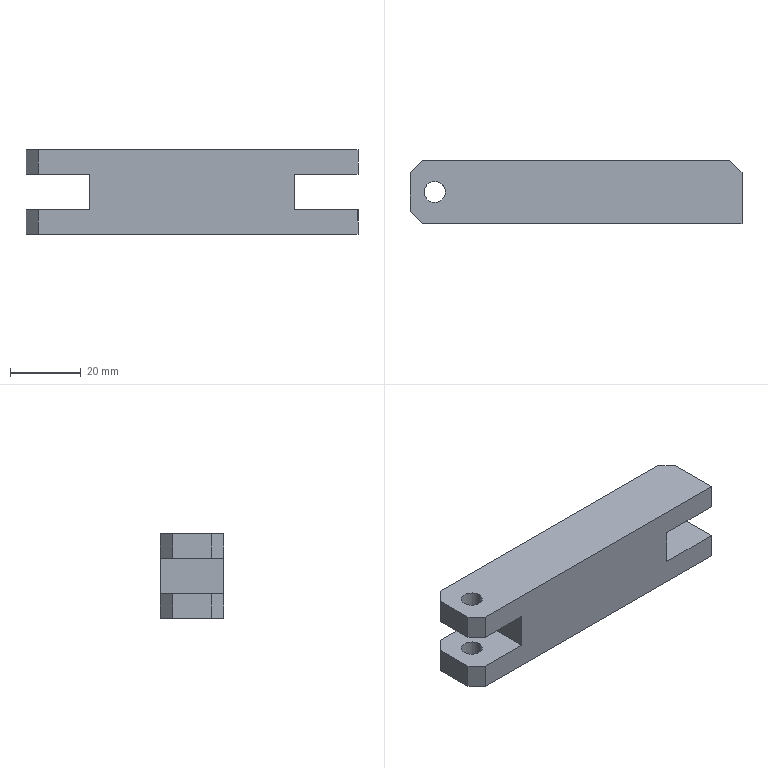Part | SolidWorks | features Chamfer 2, ICE 2, Extrusion 1 | 1 solid | 24 faces | box 94 x 18 x 24 mm | volume 33475 mm3 | plane 20 | cylinder 4 | commonest cylinder face diameters 6 x4
STEP:
#1=CARTESIAN_POINT('',(-43.,9.,5.));
#2=VERTEX_POINT('',#1);
#3=CARTESIAN_POINT('',(-37.,9.,5.));
#4=VERTEX_POINT('',#3);
#5=CARTESIAN_POINT('',(-40.,9.,5.));
#6=DIRECTION('',(0.,0.,1.));
#7=DIRECTION('',(1.,0.,0.));
#8=AXIS2_PLACEMENT_3D('',#5,#6,#7);
#9=CIRCLE('',#8,3.);
#10=EDGE_CURVE('',#2,#4,#9,.T.);
#11=ORIENTED_EDGE('',*,*,#10,.F.);
#12=CARTESIAN_POINT('',(-43.,9.,12.));
#13=VERTEX_POINT('',#12);
#14=CARTESIAN_POINT('',(-43.,9.,-58.));
#15=DIRECTION('',(0.,0.,1.));
#16=VECTOR('',#15,1000.);
#17=LINE('',#14,#16);
#18=EDGE_CURVE('',#2,#13,#17,.T.);
#19=ORIENTED_EDGE('',*,*,#18,.T.);
#20=CARTESIAN_POINT('',(-37.,9.,12.));
#21=VERTEX_POINT('',#20);
#22=CARTESIAN_POINT('',(-40.,9.,12.));
#23=DIRECTION('',(0.,0.,1.));
#24=DIRECTION('',(1.,0.,0.));
#25=AXIS2_PLACEMENT_3D('',#22,#23,#24);
#26=CIRCLE('',#25,3.);
#27=EDGE_CURVE('',#13,#21,#26,.T.);
#28=ORIENTED_EDGE('',*,*,#27,.T.);
#29=CARTESIAN_POINT('',(-37.,9.,-58.));
#30=DIRECTION('',(0.,0.,1.));
#31=VECTOR('',#30,1000.);
#32=LINE('',#29,#31);
#33=EDGE_CURVE('',#4,#21,#32,.T.);
#34=ORIENTED_EDGE('',*,*,#33,.F.);
#35=EDGE_LOOP('',(#11,#19,#28,#34));
#36=FACE_OUTER_BOUND('',#35,.T.);
#37=CARTESIAN_POINT('',(-40.,9.,-58.));
#38=DIRECTION('',(0.,0.,1.));
#39=DIRECTION('',(1.,0.,0.));
#40=AXIS2_PLACEMENT_3D('',#37,#38,#39);
#41=CYLINDRICAL_SURFACE('',#40,3.);
#42=ADVANCED_FACE('',(#36),#41,.F.);
#43=CARTESIAN_POINT('',(-43.,9.,-12.));
#44=VERTEX_POINT('',#43);
#45=CARTESIAN_POINT('',(-37.,9.,-12.));
#46=VERTEX_POINT('',#45);
#47=CARTESIAN_POINT('',(-40.,9.,-12.));
#48=DIRECTION('',(0.,0.,1.));
#49=DIRECTION('',(1.,0.,0.));
#50=AXIS2_PLACEMENT_3D('',#47,#48,#49);
#51=CIRCLE('',#50,3.);
#52=EDGE_CURVE('',#44,#46,#51,.T.);
#53=ORIENTED_EDGE('',*,*,#52,.F.);
#54=CARTESIAN_POINT('',(-43.,9.,-5.));
#55=VERTEX_POINT('',#54);
#56=CARTESIAN_POINT('',(-43.,9.,-58.));
#57=DIRECTION('',(0.,0.,1.));
#58=VECTOR('',#57,1000.);
#59=LINE('',#56,#58);
#60=EDGE_CURVE('',#44,#55,#59,.T.);
#61=ORIENTED_EDGE('',*,*,#60,.T.);
#62=CARTESIAN_POINT('',(-37.,9.,-5.));
#63=VERTEX_POINT('',#62);
#64=CARTESIAN_POINT('',(-40.,9.,-5.));
#65=DIRECTION('',(0.,0.,-1.));
#66=DIRECTION('',(-1.,0.,0.));
#67=AXIS2_PLACEMENT_3D('',#64,#65,#66);
#68=CIRCLE('',#67,3.);
#69=EDGE_CURVE('',#63,#55,#68,.T.);
#70=ORIENTED_EDGE('',*,*,#69,.F.);
#71=CARTESIAN_POINT('',(-37.,9.,-58.));
#72=DIRECTION('',(0.,0.,1.));
#73=VECTOR('',#72,1000.);
#74=LINE('',#71,#73);
#75=EDGE_CURVE('',#46,#63,#74,.T.);
#76=ORIENTED_EDGE('',*,*,#75,.F.);
#77=EDGE_LOOP('',(#53,#61,#70,#76));
#78=FACE_OUTER_BOUND('',#77,.T.);
#79=CARTESIAN_POINT('',(-40.,9.,-58.));
#80=DIRECTION('',(0.,0.,1.));
#81=DIRECTION('',(1.,0.,0.));
#82=AXIS2_PLACEMENT_3D('',#79,#80,#81);
#83=CYLINDRICAL_SURFACE('',#82,3.);
#84=ADVANCED_FACE('',(#78),#83,.F.);
#85=CARTESIAN_POINT('',(47.,0.,5.));
#86=VERTEX_POINT('',#85);
#87=CARTESIAN_POINT('',(47.,14.5,5.));
#88=VERTEX_POINT('',#87);
#89=CARTESIAN_POINT('',(47.,18.,5.));
#90=DIRECTION('',(0.,1.,0.));
#91=VECTOR('',#90,1000.);
#92=LINE('',#89,#91);
#93=EDGE_CURVE('',#86,#88,#92,.T.);
#94=ORIENTED_EDGE('',*,*,#93,.T.);
#95=CARTESIAN_POINT('',(47.,14.5,12.));
#96=VERTEX_POINT('',#95);
#97=CARTESIAN_POINT('',(47.,14.5,12.));
#98=DIRECTION('',(0.,0.,1.));
#99=VECTOR('',#98,1000.);
#100=LINE('',#97,#99);
#101=EDGE_CURVE('',#88,#96,#100,.T.);
#102=ORIENTED_EDGE('',*,*,#101,.T.);
#103=CARTESIAN_POINT('',(47.,0.,12.));
#104=VERTEX_POINT('',#103);
#105=CARTESIAN_POINT('',(47.,18.,12.));
#106=DIRECTION('',(0.,-1.,0.));
#107=VECTOR('',#106,1000.);
#108=LINE('',#105,#107);
#109=EDGE_CURVE('',#96,#104,#108,.T.);
#110=ORIENTED_EDGE('',*,*,#109,.T.);
#111=CARTESIAN_POINT('',(47.,0.,-12.));
#112=DIRECTION('',(0.,0.,-1.));
#113=VECTOR('',#112,1000.);
#114=LINE('',#111,#113);
#115=EDGE_CURVE('',#104,#86,#114,.T.);
#116=ORIENTED_EDGE('',*,*,#115,.T.);
#117=EDGE_LOOP('',(#94,#102,#110,#116));
#118=FACE_OUTER_BOUND('',#117,.T.);
#119=CARTESIAN_POINT('',(47.,18.,-12.));
#120=DIRECTION('',(-1.,0.,0.));
#121=DIRECTION('',(0.,0.,1.));
#122=AXIS2_PLACEMENT_3D('',#119,#120,#121);
#123=PLANE('',#122);
#124=ADVANCED_FACE('',(#118),#123,.F.);
#125=CARTESIAN_POINT('',(-47.,14.5,5.));
#126=VERTEX_POINT('',#125);
#127=CARTESIAN_POINT('',(-47.,3.5,5.));
#128=VERTEX_POINT('',#127);
#129=CARTESIAN_POINT('',(-47.,18.,5.));
#130=DIRECTION('',(0.,-1.,0.));
#131=VECTOR('',#130,1000.);
#132=LINE('',#129,#131);
#133=EDGE_CURVE('',#126,#128,#132,.T.);
#134=ORIENTED_EDGE('',*,*,#133,.T.);
#135=CARTESIAN_POINT('',(-47.,3.5,12.));
#136=VERTEX_POINT('',#135);
#137=CARTESIAN_POINT('',(-47.,3.5,-12.));
#138=DIRECTION('',(0.,0.,1.));
#139=VECTOR('',#138,1000.);
#140=LINE('',#137,#139);
#141=EDGE_CURVE('',#128,#136,#140,.T.);
#142=ORIENTED_EDGE('',*,*,#141,.T.);
#143=CARTESIAN_POINT('',(-47.,14.5,12.));
#144=VERTEX_POINT('',#143);
#145=CARTESIAN_POINT('',(-47.,18.,12.));
#146=DIRECTION('',(0.,-1.,0.));
#147=VECTOR('',#146,1000.);
#148=LINE('',#145,#147);
#149=EDGE_CURVE('',#144,#136,#148,.T.);
#150=ORIENTED_EDGE('',*,*,#149,.F.);
#151=CARTESIAN_POINT('',(-47.,14.5,5.));
#152=DIRECTION('',(0.,0.,-1.));
#153=VECTOR('',#152,1000.);
#154=LINE('',#151,#153);
#155=EDGE_CURVE('',#144,#126,#154,.T.);
#156=ORIENTED_EDGE('',*,*,#155,.T.);
#157=EDGE_LOOP('',(#134,#142,#150,#156));
#158=FACE_OUTER_BOUND('',#157,.T.);
#159=CARTESIAN_POINT('',(-47.,18.,-12.));
#160=DIRECTION('',(1.,0.,0.));
#161=DIRECTION('',(0.,0.,-1.));
#162=AXIS2_PLACEMENT_3D('',#159,#160,#161);
#163=PLANE('',#162);
#164=ADVANCED_FACE('',(#158),#163,.F.);
#165=CARTESIAN_POINT('',(47.,14.5,-12.));
#166=VERTEX_POINT('',#165);
#167=CARTESIAN_POINT('',(47.,0.,-12.));
#168=VERTEX_POINT('',#167);
#169=CARTESIAN_POINT('',(47.,18.,-12.));
#170=DIRECTION('',(0.,-1.,0.));
#171=VECTOR('',#170,1000.);
#172=LINE('',#169,#171);
#173=EDGE_CURVE('',#166,#168,#172,.T.);
#174=ORIENTED_EDGE('',*,*,#173,.F.);
#175=CARTESIAN_POINT('',(47.,14.5,-5.));
#176=VERTEX_POINT('',#175);
#177=CARTESIAN_POINT('',(47.,14.5,-5.));
#178=DIRECTION('',(0.,0.,1.));
#179=VECTOR('',#178,1000.);
#180=LINE('',#177,#179);
#181=EDGE_CURVE('',#166,#176,#180,.T.);
#182=ORIENTED_EDGE('',*,*,#181,.T.);
#183=CARTESIAN_POINT('',(47.,0.,-5.));
#184=VERTEX_POINT('',#183);
#185=CARTESIAN_POINT('',(47.,18.,-5.));
#186=DIRECTION('',(0.,-1.,0.));
#187=VECTOR('',#186,1000.);
#188=LINE('',#185,#187);
#189=EDGE_CURVE('',#176,#184,#188,.T.);
#190=ORIENTED_EDGE('',*,*,#189,.T.);
#191=CARTESIAN_POINT('',(47.,0.,-12.));
#192=DIRECTION('',(0.,0.,-1.));
#193=VECTOR('',#192,1000.);
#194=LINE('',#191,#193);
#195=EDGE_CURVE('',#184,#168,#194,.T.);
#196=ORIENTED_EDGE('',*,*,#195,.T.);
#197=EDGE_LOOP('',(#174,#182,#190,#196));
#198=FACE_OUTER_BOUND('',#197,.T.);
#199=CARTESIAN_POINT('',(47.,18.,-12.));
#200=DIRECTION('',(-1.,0.,0.));
#201=DIRECTION('',(0.,0.,1.));
#202=AXIS2_PLACEMENT_3D('',#199,#200,#201);
#203=PLANE('',#202);
#204=ADVANCED_FACE('',(#198),#203,.F.);
#205=CARTESIAN_POINT('',(-40.,9.,-12.));
#206=DIRECTION('',(0.,0.,1.));
#207=DIRECTION('',(1.,0.,0.));
#208=AXIS2_PLACEMENT_3D('',#205,#206,#207);
#209=CIRCLE('',#208,3.);
#210=EDGE_CURVE('',#46,#44,#209,.T.);
#211=ORIENTED_EDGE('',*,*,#210,.T.);
#212=ORIENTED_EDGE('',*,*,#52,.T.);
#213=EDGE_LOOP('',(#211,#212));
#214=FACE_BOUND('',#213,.T.);
#215=CARTESIAN_POINT('',(-43.5,0.,-12.));
#216=VERTEX_POINT('',#215);
#217=CARTESIAN_POINT('',(-47.,0.,-12.));
#218=DIRECTION('',(-1.,0.,0.));
#219=VECTOR('',#218,1000.);
#220=LINE('',#217,#219);
#221=EDGE_CURVE('',#168,#216,#220,.T.);
#222=ORIENTED_EDGE('',*,*,#221,.T.);
#223=CARTESIAN_POINT('',(-47.,3.5,-12.));
#224=VERTEX_POINT('',#223);
#225=CARTESIAN_POINT('',(-47.,3.5,-12.));
#226=DIRECTION('',(-0.7071,0.7071,0.));
#227=VECTOR('',#226,1000.);
#228=LINE('',#225,#227);
#229=EDGE_CURVE('',#216,#224,#228,.T.);
#230=ORIENTED_EDGE('',*,*,#229,.T.);
#231=CARTESIAN_POINT('',(-47.,14.5,-12.));
#232=VERTEX_POINT('',#231);
#233=CARTESIAN_POINT('',(-47.,18.,-12.));
#234=DIRECTION('',(0.,-1.,0.));
#235=VECTOR('',#234,1000.);
#236=LINE('',#233,#235);
#237=EDGE_CURVE('',#232,#224,#236,.T.);
#238=ORIENTED_EDGE('',*,*,#237,.F.);
#239=CARTESIAN_POINT('',(-43.5,18.,-12.));
#240=VERTEX_POINT('',#239);
#241=CARTESIAN_POINT('',(-43.5,18.,-12.));
#242=DIRECTION('',(0.7071,0.7071,0.));
#243=VECTOR('',#242,1000.);
#244=LINE('',#241,#243);
#245=EDGE_CURVE('',#232,#240,#244,.T.);
#246=ORIENTED_EDGE('',*,*,#245,.T.);
#247=CARTESIAN_POINT('',(43.5,18.,-12.));
#248=VERTEX_POINT('',#247);
#249=CARTESIAN_POINT('',(-47.,18.,-12.));
#250=DIRECTION('',(-1.,0.,0.));
#251=VECTOR('',#250,1000.);
#252=LINE('',#249,#251);
#253=EDGE_CURVE('',#248,#240,#252,.T.);
#254=ORIENTED_EDGE('',*,*,#253,.F.);
#255=CARTESIAN_POINT('',(43.5,18.,-12.));
#256=DIRECTION('',(0.7071,-0.7071,0.));
#257=VECTOR('',#256,1000.);
#258=LINE('',#255,#257);
#259=EDGE_CURVE('',#248,#166,#258,.T.);
#260=ORIENTED_EDGE('',*,*,#259,.T.);
#261=ORIENTED_EDGE('',*,*,#173,.T.);
#262=EDGE_LOOP('',(#222,#230,#238,#246,#254,#260,#261));
#263=FACE_OUTER_BOUND('',#262,.T.);
#264=CARTESIAN_POINT('',(-47.,18.,-12.));
#265=DIRECTION('',(0.,0.,1.));
#266=DIRECTION('',(1.,0.,0.));
#267=AXIS2_PLACEMENT_3D('',#264,#265,#266);
#268=PLANE('',#267);
#269=ADVANCED_FACE('',(#214,#263),#268,.F.);
#270=ORIENTED_EDGE('',*,*,#237,.T.);
#271=CARTESIAN_POINT('',(-47.,3.5,-5.));
#272=VERTEX_POINT('',#271);
#273=CARTESIAN_POINT('',(-47.,3.5,-12.));
#274=DIRECTION('',(0.,0.,1.));
#275=VECTOR('',#274,1000.);
#276=LINE('',#273,#275);
#277=EDGE_CURVE('',#224,#272,#276,.T.);
#278=ORIENTED_EDGE('',*,*,#277,.T.);
#279=CARTESIAN_POINT('',(-47.,14.5,-5.));
#280=VERTEX_POINT('',#279);
#281=CARTESIAN_POINT('',(-47.,18.,-5.));
#282=DIRECTION('',(0.,1.,0.));
#283=VECTOR('',#282,1000.);
#284=LINE('',#281,#283);
#285=EDGE_CURVE('',#272,#280,#284,.T.);
#286=ORIENTED_EDGE('',*,*,#285,.T.);
#287=CARTESIAN_POINT('',(-47.,14.5,-12.));
#288=DIRECTION('',(0.,0.,-1.));
#289=VECTOR('',#288,1000.);
#290=LINE('',#287,#289);
#291=EDGE_CURVE('',#280,#232,#290,.T.);
#292=ORIENTED_EDGE('',*,*,#291,.T.);
#293=EDGE_LOOP('',(#270,#278,#286,#292));
#294=FACE_OUTER_BOUND('',#293,.T.);
#295=CARTESIAN_POINT('',(-47.,18.,-12.));
#296=DIRECTION('',(1.,0.,0.));
#297=DIRECTION('',(0.,0.,-1.));
#298=AXIS2_PLACEMENT_3D('',#295,#296,#297);
#299=PLANE('',#298);
#300=ADVANCED_FACE('',(#294),#299,.F.);
#301=CARTESIAN_POINT('',(-40.,9.,12.));
#302=DIRECTION('',(0.,0.,1.));
#303=DIRECTION('',(1.,0.,0.));
#304=AXIS2_PLACEMENT_3D('',#301,#302,#303);
#305=CIRCLE('',#304,3.);
#306=EDGE_CURVE('',#21,#13,#305,.T.);
#307=ORIENTED_EDGE('',*,*,#306,.F.);
#308=ORIENTED_EDGE('',*,*,#27,.F.);
#309=EDGE_LOOP('',(#307,#308));
#310=FACE_BOUND('',#309,.T.);
#311=ORIENTED_EDGE('',*,*,#149,.T.);
#312=CARTESIAN_POINT('',(-43.5,0.,12.));
#313=VERTEX_POINT('',#312);
#314=CARTESIAN_POINT('',(-47.,3.5,12.));
#315=DIRECTION('',(0.7071,-0.7071,0.));
#316=VECTOR('',#315,1000.);
#317=LINE('',#314,#316);
#318=EDGE_CURVE('',#136,#313,#317,.T.);
#319=ORIENTED_EDGE('',*,*,#318,.T.);
#320=CARTESIAN_POINT('',(-47.,0.,12.));
#321=DIRECTION('',(1.,0.,0.));
#322=VECTOR('',#321,1000.);
#323=LINE('',#320,#322);
#324=EDGE_CURVE('',#313,#104,#323,.T.);
#325=ORIENTED_EDGE('',*,*,#324,.T.);
#326=ORIENTED_EDGE('',*,*,#109,.F.);
#327=CARTESIAN_POINT('',(43.5,18.,12.));
#328=VERTEX_POINT('',#327);
#329=CARTESIAN_POINT('',(43.5,18.,12.));
#330=DIRECTION('',(-0.7071,0.7071,0.));
#331=VECTOR('',#330,1000.);
#332=LINE('',#329,#331);
#333=EDGE_CURVE('',#96,#328,#332,.T.);
#334=ORIENTED_EDGE('',*,*,#333,.T.);
#335=CARTESIAN_POINT('',(-43.5,18.,12.));
#336=VERTEX_POINT('',#335);
#337=CARTESIAN_POINT('',(-47.,18.,12.));
#338=DIRECTION('',(1.,0.,0.));
#339=VECTOR('',#338,1000.);
#340=LINE('',#337,#339);
#341=EDGE_CURVE('',#336,#328,#340,.T.);
#342=ORIENTED_EDGE('',*,*,#341,.F.);
#343=CARTESIAN_POINT('',(-43.5,18.,12.));
#344=DIRECTION('',(-0.7071,-0.7071,0.));
#345=VECTOR('',#344,1000.);
#346=LINE('',#343,#345);
#347=EDGE_CURVE('',#336,#144,#346,.T.);
#348=ORIENTED_EDGE('',*,*,#347,.T.);
#349=EDGE_LOOP('',(#311,#319,#325,#326,#334,#342,#348));
#350=FACE_OUTER_BOUND('',#349,.T.);
#351=CARTESIAN_POINT('',(-47.,18.,12.));
#352=DIRECTION('',(0.,0.,-1.));
#353=DIRECTION('',(-1.,0.,0.));
#354=AXIS2_PLACEMENT_3D('',#351,#352,#353);
#355=PLANE('',#354);
#356=ADVANCED_FACE('',(#310,#350),#355,.F.);
#357=ORIENTED_EDGE('',*,*,#253,.T.);
#358=CARTESIAN_POINT('',(-43.5,18.,-5.));
#359=VERTEX_POINT('',#358);
#360=CARTESIAN_POINT('',(-43.5,18.,-5.));
#361=DIRECTION('',(0.,0.,1.));
#362=VECTOR('',#361,1000.);
#363=LINE('',#360,#362);
#364=EDGE_CURVE('',#240,#359,#363,.T.);
#365=ORIENTED_EDGE('',*,*,#364,.T.);
#366=CARTESIAN_POINT('',(-29.,18.,-5.));
#367=VERTEX_POINT('',#366);
#368=CARTESIAN_POINT('',(-65.,18.,-5.));
#369=DIRECTION('',(-1.,0.,0.));
#370=VECTOR('',#369,1000.);
#371=LINE('',#368,#370);
#372=EDGE_CURVE('',#367,#359,#371,.T.);
#373=ORIENTED_EDGE('',*,*,#372,.F.);
#374=CARTESIAN_POINT('',(-29.,18.,5.));
#375=VERTEX_POINT('',#374);
#376=CARTESIAN_POINT('',(-29.,18.,-5.));
#377=DIRECTION('',(0.,0.,-1.));
#378=VECTOR('',#377,1000.);
#379=LINE('',#376,#378);
#380=EDGE_CURVE('',#375,#367,#379,.T.);
#381=ORIENTED_EDGE('',*,*,#380,.F.);
#382=CARTESIAN_POINT('',(-43.5,18.,5.));
#383=VERTEX_POINT('',#382);
#384=CARTESIAN_POINT('',(-65.,18.,5.));
#385=DIRECTION('',(1.,0.,0.));
#386=VECTOR('',#385,1000.);
#387=LINE('',#384,#386);
#388=EDGE_CURVE('',#383,#375,#387,.T.);
#389=ORIENTED_EDGE('',*,*,#388,.F.);
#390=CARTESIAN_POINT('',(-43.5,18.,12.));
#391=DIRECTION('',(0.,0.,1.));
#392=VECTOR('',#391,1000.);
#393=LINE('',#390,#392);
#394=EDGE_CURVE('',#383,#336,#393,.T.);
#395=ORIENTED_EDGE('',*,*,#394,.T.);
#396=ORIENTED_EDGE('',*,*,#341,.T.);
#397=CARTESIAN_POINT('',(43.5,18.,5.));
#398=VERTEX_POINT('',#397);
#399=CARTESIAN_POINT('',(43.5,18.,5.));
#400=DIRECTION('',(0.,0.,-1.));
#401=VECTOR('',#400,1000.);
#402=LINE('',#399,#401);
#403=EDGE_CURVE('',#328,#398,#402,.T.);
#404=ORIENTED_EDGE('',*,*,#403,.T.);
#405=CARTESIAN_POINT('',(29.,18.,5.));
#406=VERTEX_POINT('',#405);
#407=CARTESIAN_POINT('',(65.,18.,5.));
#408=DIRECTION('',(1.,0.,0.));
#409=VECTOR('',#408,1000.);
#410=LINE('',#407,#409);
#411=EDGE_CURVE('',#406,#398,#410,.T.);
#412=ORIENTED_EDGE('',*,*,#411,.F.);
#413=CARTESIAN_POINT('',(29.,18.,-5.));
#414=VERTEX_POINT('',#413);
#415=CARTESIAN_POINT('',(29.,18.,-5.));
#416=DIRECTION('',(0.,0.,1.));
#417=VECTOR('',#416,1000.);
#418=LINE('',#415,#417);
#419=EDGE_CURVE('',#414,#406,#418,.T.);
#420=ORIENTED_EDGE('',*,*,#419,.F.);
#421=CARTESIAN_POINT('',(43.5,18.,-5.));
#422=VERTEX_POINT('',#421);
#423=CARTESIAN_POINT('',(65.,18.,-5.));
#424=DIRECTION('',(-1.,0.,0.));
#425=VECTOR('',#424,1000.);
#426=LINE('',#423,#425);
#427=EDGE_CURVE('',#422,#414,#426,.T.);
#428=ORIENTED_EDGE('',*,*,#427,.F.);
#429=CARTESIAN_POINT('',(43.5,18.,-12.));
#430=DIRECTION('',(0.,0.,-1.));
#431=VECTOR('',#430,1000.);
#432=LINE('',#429,#431);
#433=EDGE_CURVE('',#422,#248,#432,.T.);
#434=ORIENTED_EDGE('',*,*,#433,.T.);
#435=EDGE_LOOP('',(#357,#365,#373,#381,#389,#395,#396,#404,#412,#420,#428,#434));
#436=FACE_OUTER_BOUND('',#435,.T.);
#437=CARTESIAN_POINT('',(47.,18.,12.));
#438=DIRECTION('',(0.,1.,0.));
#439=DIRECTION('',(0.,0.,1.));
#440=AXIS2_PLACEMENT_3D('',#437,#438,#439);
#441=PLANE('',#440);
#442=ADVANCED_FACE('',(#436),#441,.T.);
#443=ORIENTED_EDGE('',*,*,#324,.F.);
#444=CARTESIAN_POINT('',(-43.5,0.,5.));
#445=VERTEX_POINT('',#444);
#446=CARTESIAN_POINT('',(-43.5,0.,12.));
#447=DIRECTION('',(0.,0.,-1.));
#448=VECTOR('',#447,1000.);
#449=LINE('',#446,#448);
#450=EDGE_CURVE('',#313,#445,#449,.T.);
#451=ORIENTED_EDGE('',*,*,#450,.T.);
#452=CARTESIAN_POINT('',(-29.,0.,5.));
#453=VERTEX_POINT('',#452);
#454=CARTESIAN_POINT('',(47.,0.,5.));
#455=DIRECTION('',(1.,0.,0.));
#456=VECTOR('',#455,1000.);
#457=LINE('',#454,#456);
#458=EDGE_CURVE('',#445,#453,#457,.T.);
#459=ORIENTED_EDGE('',*,*,#458,.T.);
#460=CARTESIAN_POINT('',(-29.,0.,-5.));
#461=VERTEX_POINT('',#460);
#462=CARTESIAN_POINT('',(-29.,0.,12.));
#463=DIRECTION('',(0.,0.,-1.));
#464=VECTOR('',#463,1000.);
#465=LINE('',#462,#464);
#466=EDGE_CURVE('',#453,#461,#465,.T.);
#467=ORIENTED_EDGE('',*,*,#466,.T.);
#468=CARTESIAN_POINT('',(-43.5,0.,-5.));
#469=VERTEX_POINT('',#468);
#470=CARTESIAN_POINT('',(47.,0.,-5.));
#471=DIRECTION('',(-1.,0.,0.));
#472=VECTOR('',#471,1000.);
#473=LINE('',#470,#472);
#474=EDGE_CURVE('',#461,#469,#473,.T.);
#475=ORIENTED_EDGE('',*,*,#474,.T.);
#476=CARTESIAN_POINT('',(-43.5,0.,12.));
#477=DIRECTION('',(0.,0.,-1.));
#478=VECTOR('',#477,1000.);
#479=LINE('',#476,#478);
#480=EDGE_CURVE('',#469,#216,#479,.T.);
#481=ORIENTED_EDGE('',*,*,#480,.T.);
#482=ORIENTED_EDGE('',*,*,#221,.F.);
#483=ORIENTED_EDGE('',*,*,#195,.F.);
#484=CARTESIAN_POINT('',(29.,0.,-5.));
#485=VERTEX_POINT('',#484);
#486=CARTESIAN_POINT('',(47.,0.,-5.));
#487=DIRECTION('',(-1.,0.,0.));
#488=VECTOR('',#487,1000.);
#489=LINE('',#486,#488);
#490=EDGE_CURVE('',#184,#485,#489,.T.);
#491=ORIENTED_EDGE('',*,*,#490,.T.);
#492=CARTESIAN_POINT('',(29.,0.,5.));
#493=VERTEX_POINT('',#492);
#494=CARTESIAN_POINT('',(29.,0.,12.));
#495=DIRECTION('',(0.,0.,1.));
#496=VECTOR('',#495,1000.);
#497=LINE('',#494,#496);
#498=EDGE_CURVE('',#485,#493,#497,.T.);
#499=ORIENTED_EDGE('',*,*,#498,.T.);
#500=CARTESIAN_POINT('',(47.,0.,5.));
#501=DIRECTION('',(1.,0.,0.));
#502=VECTOR('',#501,1000.);
#503=LINE('',#500,#502);
#504=EDGE_CURVE('',#493,#86,#503,.T.);
#505=ORIENTED_EDGE('',*,*,#504,.T.);
#506=ORIENTED_EDGE('',*,*,#115,.F.);
#507=EDGE_LOOP('',(#443,#451,#459,#467,#475,#481,#482,#483,#491,#499,#505,#506));
#508=FACE_OUTER_BOUND('',#507,.T.);
#509=CARTESIAN_POINT('',(47.,0.,12.));
#510=DIRECTION('',(0.,1.,0.));
#511=DIRECTION('',(0.,0.,1.));
#512=AXIS2_PLACEMENT_3D('',#509,#510,#511);
#513=PLANE('',#512);
#514=ADVANCED_FACE('',(#508),#513,.F.);
#515=CARTESIAN_POINT('',(-29.,-52.,5.));
#516=DIRECTION('',(0.,1.,0.));
#517=VECTOR('',#516,1000.);
#518=LINE('',#515,#517);
#519=EDGE_CURVE('',#453,#375,#518,.T.);
#520=ORIENTED_EDGE('',*,*,#519,.T.);
#521=ORIENTED_EDGE('',*,*,#380,.T.);
#522=CARTESIAN_POINT('',(-29.,-52.,-5.));
#523=DIRECTION('',(0.,1.,0.));
#524=VECTOR('',#523,1000.);
#525=LINE('',#522,#524);
#526=EDGE_CURVE('',#461,#367,#525,.T.);
#527=ORIENTED_EDGE('',*,*,#526,.F.);
#528=ORIENTED_EDGE('',*,*,#466,.F.);
#529=EDGE_LOOP('',(#520,#521,#527,#528));
#530=FACE_OUTER_BOUND('',#529,.T.);
#531=CARTESIAN_POINT('',(-29.,-52.,-5.));
#532=DIRECTION('',(1.,0.,0.));
#533=DIRECTION('',(0.,0.,-1.));
#534=AXIS2_PLACEMENT_3D('',#531,#532,#533);
#535=PLANE('',#534);
#536=ADVANCED_FACE('',(#530),#535,.F.);
#537=CARTESIAN_POINT('',(-40.,9.,5.));
#538=DIRECTION('',(0.,0.,1.));
#539=DIRECTION('',(1.,0.,0.));
#540=AXIS2_PLACEMENT_3D('',#537,#538,#539);
#541=CIRCLE('',#540,3.);
#542=EDGE_CURVE('',#4,#2,#541,.T.);
#543=ORIENTED_EDGE('',*,*,#542,.T.);
#544=ORIENTED_EDGE('',*,*,#10,.T.);
#545=EDGE_LOOP('',(#543,#544));
#546=FACE_BOUND('',#545,.T.);
#547=ORIENTED_EDGE('',*,*,#458,.F.);
#548=CARTESIAN_POINT('',(-47.,3.5,5.));
#549=DIRECTION('',(-0.7071,0.7071,0.));
#550=VECTOR('',#549,1000.);
#551=LINE('',#548,#550);
#552=EDGE_CURVE('',#445,#128,#551,.T.);
#553=ORIENTED_EDGE('',*,*,#552,.T.);
#554=ORIENTED_EDGE('',*,*,#133,.F.);
#555=CARTESIAN_POINT('',(-43.5,18.,5.));
#556=DIRECTION('',(0.7071,0.7071,0.));
#557=VECTOR('',#556,1000.);
#558=LINE('',#555,#557);
#559=EDGE_CURVE('',#126,#383,#558,.T.);
#560=ORIENTED_EDGE('',*,*,#559,.T.);
#561=ORIENTED_EDGE('',*,*,#388,.T.);
#562=ORIENTED_EDGE('',*,*,#519,.F.);
#563=EDGE_LOOP('',(#547,#553,#554,#560,#561,#562));
#564=FACE_OUTER_BOUND('',#563,.T.);
#565=CARTESIAN_POINT('',(-65.,-52.,5.));
#566=DIRECTION('',(0.,0.,1.));
#567=DIRECTION('',(1.,0.,0.));
#568=AXIS2_PLACEMENT_3D('',#565,#566,#567);
#569=PLANE('',#568);
#570=ADVANCED_FACE('',(#546,#564),#569,.F.);
#571=ORIENTED_EDGE('',*,*,#69,.T.);
#572=CARTESIAN_POINT('',(-40.,9.,-5.));
#573=DIRECTION('',(0.,0.,-1.));
#574=DIRECTION('',(-1.,0.,0.));
#575=AXIS2_PLACEMENT_3D('',#572,#573,#574);
#576=CIRCLE('',#575,3.);
#577=EDGE_CURVE('',#55,#63,#576,.T.);
#578=ORIENTED_EDGE('',*,*,#577,.T.);
#579=EDGE_LOOP('',(#571,#578));
#580=FACE_BOUND('',#579,.T.);
#581=ORIENTED_EDGE('',*,*,#285,.F.);
#582=CARTESIAN_POINT('',(-47.,3.5,-5.));
#583=DIRECTION('',(0.7071,-0.7071,0.));
#584=VECTOR('',#583,1000.);
#585=LINE('',#582,#584);
#586=EDGE_CURVE('',#272,#469,#585,.T.);
#587=ORIENTED_EDGE('',*,*,#586,.T.);
#588=ORIENTED_EDGE('',*,*,#474,.F.);
#589=ORIENTED_EDGE('',*,*,#526,.T.);
#590=ORIENTED_EDGE('',*,*,#372,.T.);
#591=CARTESIAN_POINT('',(-43.5,18.,-5.));
#592=DIRECTION('',(-0.7071,-0.7071,0.));
#593=VECTOR('',#592,1000.);
#594=LINE('',#591,#593);
#595=EDGE_CURVE('',#359,#280,#594,.T.);
#596=ORIENTED_EDGE('',*,*,#595,.T.);
#597=EDGE_LOOP('',(#581,#587,#588,#589,#590,#596));
#598=FACE_OUTER_BOUND('',#597,.T.);
#599=CARTESIAN_POINT('',(-65.,-52.,-5.));
#600=DIRECTION('',(0.,0.,-1.));
#601=DIRECTION('',(-1.,0.,0.));
#602=AXIS2_PLACEMENT_3D('',#599,#600,#601);
#603=PLANE('',#602);
#604=ADVANCED_FACE('',(#580,#598),#603,.F.);
#605=ORIENTED_EDGE('',*,*,#411,.T.);
#606=CARTESIAN_POINT('',(43.5,18.,5.));
#607=DIRECTION('',(0.7071,-0.7071,0.));
#608=VECTOR('',#607,1000.);
#609=LINE('',#606,#608);
#610=EDGE_CURVE('',#398,#88,#609,.T.);
#611=ORIENTED_EDGE('',*,*,#610,.T.);
#612=ORIENTED_EDGE('',*,*,#93,.F.);
#613=ORIENTED_EDGE('',*,*,#504,.F.);
#614=CARTESIAN_POINT('',(29.,-52.,5.));
#615=DIRECTION('',(0.,1.,0.));
#616=VECTOR('',#615,1000.);
#617=LINE('',#614,#616);
#618=EDGE_CURVE('',#493,#406,#617,.T.);
#619=ORIENTED_EDGE('',*,*,#618,.T.);
#620=EDGE_LOOP('',(#605,#611,#612,#613,#619));
#621=FACE_OUTER_BOUND('',#620,.T.);
#622=CARTESIAN_POINT('',(65.,-52.,5.));
#623=DIRECTION('',(0.,0.,1.));
#624=DIRECTION('',(1.,0.,0.));
#625=AXIS2_PLACEMENT_3D('',#622,#623,#624);
#626=PLANE('',#625);
#627=ADVANCED_FACE('',(#621),#626,.F.);
#628=CARTESIAN_POINT('',(29.,-52.,-5.));
#629=DIRECTION('',(0.,1.,0.));
#630=VECTOR('',#629,1000.);
#631=LINE('',#628,#630);
#632=EDGE_CURVE('',#485,#414,#631,.T.);
#633=ORIENTED_EDGE('',*,*,#632,.T.);
#634=ORIENTED_EDGE('',*,*,#419,.T.);
#635=ORIENTED_EDGE('',*,*,#618,.F.);
#636=ORIENTED_EDGE('',*,*,#498,.F.);
#637=EDGE_LOOP('',(#633,#634,#635,#636));
#638=FACE_OUTER_BOUND('',#637,.T.);
#639=CARTESIAN_POINT('',(29.,-52.,-5.));
#640=DIRECTION('',(-1.,0.,0.));
#641=DIRECTION('',(0.,0.,1.));
#642=AXIS2_PLACEMENT_3D('',#639,#640,#641);
#643=PLANE('',#642);
#644=ADVANCED_FACE('',(#638),#643,.F.);
#645=ORIENTED_EDGE('',*,*,#189,.F.);
#646=CARTESIAN_POINT('',(43.5,18.,-5.));
#647=DIRECTION('',(-0.7071,0.7071,0.));
#648=VECTOR('',#647,1000.);
#649=LINE('',#646,#648);
#650=EDGE_CURVE('',#176,#422,#649,.T.);
#651=ORIENTED_EDGE('',*,*,#650,.T.);
#652=ORIENTED_EDGE('',*,*,#427,.T.);
#653=ORIENTED_EDGE('',*,*,#632,.F.);
#654=ORIENTED_EDGE('',*,*,#490,.F.);
#655=EDGE_LOOP('',(#645,#651,#652,#653,#654));
#656=FACE_OUTER_BOUND('',#655,.T.);
#657=CARTESIAN_POINT('',(65.,-52.,-5.));
#658=DIRECTION('',(0.,0.,-1.));
#659=DIRECTION('',(-1.,0.,0.));
#660=AXIS2_PLACEMENT_3D('',#657,#658,#659);
#661=PLANE('',#660);
#662=ADVANCED_FACE('',(#656),#661,.F.);
#663=ORIENTED_EDGE('',*,*,#333,.F.);
#664=ORIENTED_EDGE('',*,*,#101,.F.);
#665=ORIENTED_EDGE('',*,*,#610,.F.);
#666=ORIENTED_EDGE('',*,*,#403,.F.);
#667=EDGE_LOOP('',(#663,#664,#665,#666));
#668=FACE_OUTER_BOUND('',#667,.T.);
#669=CARTESIAN_POINT('',(43.5,18.,12.));
#670=DIRECTION('',(0.7071,0.7071,0.));
#671=DIRECTION('',(-0.7071,0.7071,0.));
#672=AXIS2_PLACEMENT_3D('',#669,#670,#671);
#673=PLANE('',#672);
#674=ADVANCED_FACE('',(#668),#673,.T.);
#675=ORIENTED_EDGE('',*,*,#650,.F.);
#676=ORIENTED_EDGE('',*,*,#181,.F.);
#677=ORIENTED_EDGE('',*,*,#259,.F.);
#678=ORIENTED_EDGE('',*,*,#433,.F.);
#679=EDGE_LOOP('',(#675,#676,#677,#678));
#680=FACE_OUTER_BOUND('',#679,.T.);
#681=CARTESIAN_POINT('',(43.5,18.,12.));
#682=DIRECTION('',(0.7071,0.7071,0.));
#683=DIRECTION('',(-0.7071,0.7071,0.));
#684=AXIS2_PLACEMENT_3D('',#681,#682,#683);
#685=PLANE('',#684);
#686=ADVANCED_FACE('',(#680),#685,.T.);
#687=ORIENTED_EDGE('',*,*,#552,.F.);
#688=ORIENTED_EDGE('',*,*,#450,.F.);
#689=ORIENTED_EDGE('',*,*,#318,.F.);
#690=ORIENTED_EDGE('',*,*,#141,.F.);
#691=EDGE_LOOP('',(#687,#688,#689,#690));
#692=FACE_OUTER_BOUND('',#691,.T.);
#693=CARTESIAN_POINT('',(-47.,3.5,-12.));
#694=DIRECTION('',(0.7071,0.7071,0.));
#695=DIRECTION('',(-0.7071,0.7071,0.));
#696=AXIS2_PLACEMENT_3D('',#693,#694,#695);
#697=PLANE('',#696);
#698=ADVANCED_FACE('',(#692),#697,.F.);
#699=ORIENTED_EDGE('',*,*,#229,.F.);
#700=ORIENTED_EDGE('',*,*,#480,.F.);
#701=ORIENTED_EDGE('',*,*,#586,.F.);
#702=ORIENTED_EDGE('',*,*,#277,.F.);
#703=EDGE_LOOP('',(#699,#700,#701,#702));
#704=FACE_OUTER_BOUND('',#703,.T.);
#705=CARTESIAN_POINT('',(-47.,3.5,-12.));
#706=DIRECTION('',(0.7071,0.7071,0.));
#707=DIRECTION('',(-0.7071,0.7071,0.));
#708=AXIS2_PLACEMENT_3D('',#705,#706,#707);
#709=PLANE('',#708);
#710=ADVANCED_FACE('',(#704),#709,.F.);
#711=ORIENTED_EDGE('',*,*,#245,.F.);
#712=ORIENTED_EDGE('',*,*,#291,.F.);
#713=ORIENTED_EDGE('',*,*,#595,.F.);
#714=ORIENTED_EDGE('',*,*,#364,.F.);
#715=EDGE_LOOP('',(#711,#712,#713,#714));
#716=FACE_OUTER_BOUND('',#715,.T.);
#717=CARTESIAN_POINT('',(-43.5,18.,12.));
#718=DIRECTION('',(-0.7071,0.7071,0.));
#719=DIRECTION('',(-0.7071,-0.7071,0.));
#720=AXIS2_PLACEMENT_3D('',#717,#718,#719);
#721=PLANE('',#720);
#722=ADVANCED_FACE('',(#716),#721,.T.);
#723=ORIENTED_EDGE('',*,*,#559,.F.);
#724=ORIENTED_EDGE('',*,*,#155,.F.);
#725=ORIENTED_EDGE('',*,*,#347,.F.);
#726=ORIENTED_EDGE('',*,*,#394,.F.);
#727=EDGE_LOOP('',(#723,#724,#725,#726));
#728=FACE_OUTER_BOUND('',#727,.T.);
#729=CARTESIAN_POINT('',(-43.5,18.,12.));
#730=DIRECTION('',(-0.7071,0.7071,0.));
#731=DIRECTION('',(-0.7071,-0.7071,0.));
#732=AXIS2_PLACEMENT_3D('',#729,#730,#731);
#733=PLANE('',#732);
#734=ADVANCED_FACE('',(#728),#733,.T.);
#735=ORIENTED_EDGE('',*,*,#60,.F.);
#736=ORIENTED_EDGE('',*,*,#210,.F.);
#737=ORIENTED_EDGE('',*,*,#75,.T.);
#738=ORIENTED_EDGE('',*,*,#577,.F.);
#739=EDGE_LOOP('',(#735,#736,#737,#738));
#740=FACE_OUTER_BOUND('',#739,.T.);
#741=CARTESIAN_POINT('',(-40.,9.,-58.));
#742=DIRECTION('',(0.,0.,1.));
#743=DIRECTION('',(1.,0.,0.));
#744=AXIS2_PLACEMENT_3D('',#741,#742,#743);
#745=CYLINDRICAL_SURFACE('',#744,3.);
#746=ADVANCED_FACE('',(#740),#745,.F.);
#747=ORIENTED_EDGE('',*,*,#18,.F.);
#748=ORIENTED_EDGE('',*,*,#542,.F.);
#749=ORIENTED_EDGE('',*,*,#33,.T.);
#750=ORIENTED_EDGE('',*,*,#306,.T.);
#751=EDGE_LOOP('',(#747,#748,#749,#750));
#752=FACE_OUTER_BOUND('',#751,.T.);
#753=CARTESIAN_POINT('',(-40.,9.,-58.));
#754=DIRECTION('',(0.,0.,1.));
#755=DIRECTION('',(1.,0.,0.));
#756=AXIS2_PLACEMENT_3D('',#753,#754,#755);
#757=CYLINDRICAL_SURFACE('',#756,3.);
#758=ADVANCED_FACE('',(#752),#757,.F.);
#759=CLOSED_SHELL('',(#42,#84,#124,#164,#204,#269,#300,#356,#442,#514,#536,#570,#604,#627,#644,#662,#674,#686,#698,#710,#722,#734,#746,#758));
#760=MANIFOLD_SOLID_BREP('',#759);
#761=CARTESIAN_POINT('',(0.,0.,0.));
#762=DIRECTION('',(0.,0.,1.));
#763=DIRECTION('',(1.,0.,0.));
#764=AXIS2_PLACEMENT_3D('',#761,#762,#763);
#765=(LENGTH_UNIT()NAMED_UNIT(*)SI_UNIT(.MILLI.,.METRE.));
#766=UNCERTAINTY_MEASURE_WITH_UNIT(LENGTH_MEASURE(0.00001),#765,'','');
#767=(NAMED_UNIT(*)PLANE_ANGLE_UNIT()SI_UNIT($,.RADIAN.));
#768=(NAMED_UNIT(*)SI_UNIT($,.STERADIAN.)SOLID_ANGLE_UNIT());
#769=(GEOMETRIC_REPRESENTATION_CONTEXT(3)GLOBAL_UNCERTAINTY_ASSIGNED_CONTEXT((#766))GLOBAL_UNIT_ASSIGNED_CONTEXT((#765,#767,#768))REPRESENTATION_CONTEXT('',''));
#770=ADVANCED_BREP_SHAPE_REPRESENTATION('',(#760,#764),#769);